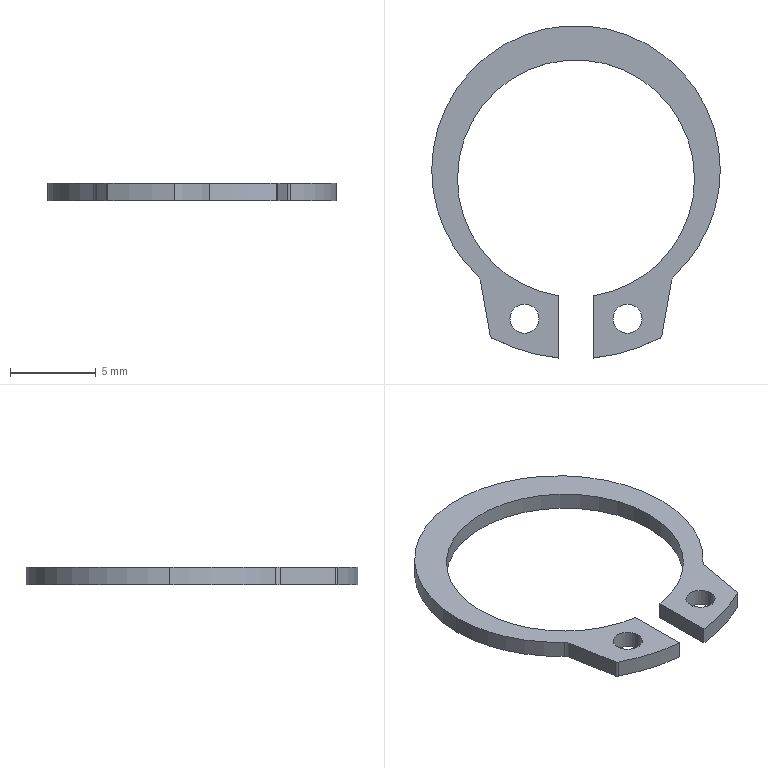Part | SolidWorks | features Extrusion 1 | 1 solid | 22 faces | box 16.8 x 19.352 x 1 mm | volume 89.212 mm3 | cylinder 16 | plane 6 | commonest cylinder face diameters 1.7 x4 13.8 x3 16.8 x3 0.4 x2 1 x2 21 x2
STEP:
#1=CARTESIAN_POINT('',(2.15,-8.666,0.5));
#2=VERTEX_POINT('',#1);
#3=CARTESIAN_POINT('',(3.85,-8.666,0.5));
#4=VERTEX_POINT('',#3);
#5=CARTESIAN_POINT('',(3.,-8.666,0.5));
#6=DIRECTION('',(0.,0.,1.));
#7=DIRECTION('',(-1.,0.,0.));
#8=AXIS2_PLACEMENT_3D('',#5,#6,#7);
#9=CIRCLE('',#8,0.85);
#10=EDGE_CURVE('',#2,#4,#9,.T.);
#11=ORIENTED_EDGE('',*,*,#10,.T.);
#12=CARTESIAN_POINT('',(3.85,-8.666,-0.5));
#13=VERTEX_POINT('',#12);
#14=CARTESIAN_POINT('',(3.85,-8.666,0.5));
#15=DIRECTION('',(0.,0.,-1.));
#16=VECTOR('',#15,1000.);
#17=LINE('',#14,#16);
#18=EDGE_CURVE('',#4,#13,#17,.T.);
#19=ORIENTED_EDGE('',*,*,#18,.T.);
#20=CARTESIAN_POINT('',(2.15,-8.666,-0.5));
#21=VERTEX_POINT('',#20);
#22=CARTESIAN_POINT('',(3.,-8.666,-0.5));
#23=DIRECTION('',(0.,0.,1.));
#24=DIRECTION('',(-1.,0.,0.));
#25=AXIS2_PLACEMENT_3D('',#22,#23,#24);
#26=CIRCLE('',#25,0.85);
#27=EDGE_CURVE('',#21,#13,#26,.T.);
#28=ORIENTED_EDGE('',*,*,#27,.F.);
#29=CARTESIAN_POINT('',(2.15,-8.666,0.5));
#30=DIRECTION('',(0.,0.,-1.));
#31=VECTOR('',#30,1000.);
#32=LINE('',#29,#31);
#33=EDGE_CURVE('',#2,#21,#32,.T.);
#34=ORIENTED_EDGE('',*,*,#33,.F.);
#35=EDGE_LOOP('',(#11,#19,#28,#34));
#36=FACE_OUTER_BOUND('',#35,.T.);
#37=CARTESIAN_POINT('',(3.,-8.666,0.5));
#38=DIRECTION('',(0.,0.,-1.));
#39=DIRECTION('',(-1.,0.,0.));
#40=AXIS2_PLACEMENT_3D('',#37,#38,#39);
#41=CYLINDRICAL_SURFACE('',#40,0.85);
#42=ADVANCED_FACE('',(#36),#41,.F.);
#43=CARTESIAN_POINT('',(-3.85,-8.666,0.5));
#44=VERTEX_POINT('',#43);
#45=CARTESIAN_POINT('',(-2.15,-8.666,0.5));
#46=VERTEX_POINT('',#45);
#47=CARTESIAN_POINT('',(-3.,-8.666,0.5));
#48=DIRECTION('',(0.,0.,1.));
#49=DIRECTION('',(1.,0.,0.));
#50=AXIS2_PLACEMENT_3D('',#47,#48,#49);
#51=CIRCLE('',#50,0.85);
#52=EDGE_CURVE('',#44,#46,#51,.T.);
#53=ORIENTED_EDGE('',*,*,#52,.T.);
#54=CARTESIAN_POINT('',(-2.15,-8.666,-0.5));
#55=VERTEX_POINT('',#54);
#56=CARTESIAN_POINT('',(-2.15,-8.666,0.5));
#57=DIRECTION('',(0.,0.,-1.));
#58=VECTOR('',#57,1000.);
#59=LINE('',#56,#58);
#60=EDGE_CURVE('',#46,#55,#59,.T.);
#61=ORIENTED_EDGE('',*,*,#60,.T.);
#62=CARTESIAN_POINT('',(-3.85,-8.666,-0.5));
#63=VERTEX_POINT('',#62);
#64=CARTESIAN_POINT('',(-3.,-8.666,-0.5));
#65=DIRECTION('',(0.,0.,1.));
#66=DIRECTION('',(1.,0.,0.));
#67=AXIS2_PLACEMENT_3D('',#64,#65,#66);
#68=CIRCLE('',#67,0.85);
#69=EDGE_CURVE('',#63,#55,#68,.T.);
#70=ORIENTED_EDGE('',*,*,#69,.F.);
#71=CARTESIAN_POINT('',(-3.85,-8.666,0.5));
#72=DIRECTION('',(0.,0.,-1.));
#73=VECTOR('',#72,1000.);
#74=LINE('',#71,#73);
#75=EDGE_CURVE('',#44,#63,#74,.T.);
#76=ORIENTED_EDGE('',*,*,#75,.F.);
#77=EDGE_LOOP('',(#53,#61,#70,#76));
#78=FACE_OUTER_BOUND('',#77,.T.);
#79=CARTESIAN_POINT('',(-3.,-8.666,0.5));
#80=DIRECTION('',(0.,0.,-1.));
#81=DIRECTION('',(-1.,0.,0.));
#82=AXIS2_PLACEMENT_3D('',#79,#80,#81);
#83=CYLINDRICAL_SURFACE('',#82,0.85);
#84=ADVANCED_FACE('',(#78),#83,.F.);
#85=CARTESIAN_POINT('',(8.4,0.,0.5));
#86=VERTEX_POINT('',#85);
#87=CARTESIAN_POINT('',(-8.4,0.,0.5));
#88=VERTEX_POINT('',#87);
#89=CARTESIAN_POINT('',(0.,0.,0.5));
#90=DIRECTION('',(0.,0.,1.));
#91=DIRECTION('',(1.,0.,0.));
#92=AXIS2_PLACEMENT_3D('',#89,#90,#91);
#93=CIRCLE('',#92,8.4);
#94=EDGE_CURVE('',#86,#88,#93,.T.);
#95=ORIENTED_EDGE('',*,*,#94,.F.);
#96=CARTESIAN_POINT('',(8.4,0.,-0.5));
#97=VERTEX_POINT('',#96);
#98=CARTESIAN_POINT('',(8.4,0.,0.5));
#99=DIRECTION('',(0.,0.,-1.));
#100=VECTOR('',#99,1000.);
#101=LINE('',#98,#100);
#102=EDGE_CURVE('',#86,#97,#101,.T.);
#103=ORIENTED_EDGE('',*,*,#102,.T.);
#104=CARTESIAN_POINT('',(-8.4,0.,-0.5));
#105=VERTEX_POINT('',#104);
#106=CARTESIAN_POINT('',(0.,0.,-0.5));
#107=DIRECTION('',(0.,0.,1.));
#108=DIRECTION('',(1.,0.,0.));
#109=AXIS2_PLACEMENT_3D('',#106,#107,#108);
#110=CIRCLE('',#109,8.4);
#111=EDGE_CURVE('',#97,#105,#110,.T.);
#112=ORIENTED_EDGE('',*,*,#111,.T.);
#113=CARTESIAN_POINT('',(-8.4,0.,0.5));
#114=DIRECTION('',(0.,0.,-1.));
#115=VECTOR('',#114,1000.);
#116=LINE('',#113,#115);
#117=EDGE_CURVE('',#88,#105,#116,.T.);
#118=ORIENTED_EDGE('',*,*,#117,.F.);
#119=EDGE_LOOP('',(#95,#103,#112,#118));
#120=FACE_OUTER_BOUND('',#119,.T.);
#121=CARTESIAN_POINT('',(0.,0.,0.5));
#122=DIRECTION('',(0.,0.,-1.));
#123=DIRECTION('',(-1.,0.,0.));
#124=AXIS2_PLACEMENT_3D('',#121,#122,#123);
#125=CYLINDRICAL_SURFACE('',#124,8.4);
#126=ADVANCED_FACE('',(#120),#125,.T.);
#127=CARTESIAN_POINT('',(-5.719,-6.153,0.5));
#128=VERTEX_POINT('',#127);
#129=CARTESIAN_POINT('',(0.,0.,0.5));
#130=DIRECTION('',(0.,0.,1.));
#131=DIRECTION('',(1.,0.,0.));
#132=AXIS2_PLACEMENT_3D('',#129,#130,#131);
#133=CIRCLE('',#132,8.4);
#134=EDGE_CURVE('',#88,#128,#133,.T.);
#135=ORIENTED_EDGE('',*,*,#134,.F.);
#136=ORIENTED_EDGE('',*,*,#117,.T.);
#137=CARTESIAN_POINT('',(-5.719,-6.153,-0.5));
#138=VERTEX_POINT('',#137);
#139=CARTESIAN_POINT('',(0.,0.,-0.5));
#140=DIRECTION('',(0.,0.,1.));
#141=DIRECTION('',(1.,0.,0.));
#142=AXIS2_PLACEMENT_3D('',#139,#140,#141);
#143=CIRCLE('',#142,8.4);
#144=EDGE_CURVE('',#105,#138,#143,.T.);
#145=ORIENTED_EDGE('',*,*,#144,.T.);
#146=CARTESIAN_POINT('',(-5.719,-6.153,0.5));
#147=DIRECTION('',(0.,0.,-1.));
#148=VECTOR('',#147,1000.);
#149=LINE('',#146,#148);
#150=EDGE_CURVE('',#128,#138,#149,.T.);
#151=ORIENTED_EDGE('',*,*,#150,.F.);
#152=EDGE_LOOP('',(#135,#136,#145,#151));
#153=FACE_OUTER_BOUND('',#152,.T.);
#154=CARTESIAN_POINT('',(0.,0.,0.5));
#155=DIRECTION('',(0.,0.,-1.));
#156=DIRECTION('',(-1.,0.,0.));
#157=AXIS2_PLACEMENT_3D('',#154,#155,#156);
#158=CYLINDRICAL_SURFACE('',#157,8.4);
#159=ADVANCED_FACE('',(#153),#158,.T.);
#160=CARTESIAN_POINT('',(6.9,-0.5,0.5));
#161=VERTEX_POINT('',#160);
#162=CARTESIAN_POINT('',(1.,-7.327,0.5));
#163=VERTEX_POINT('',#162);
#164=CARTESIAN_POINT('',(0.,-0.5,0.5));
#165=DIRECTION('',(0.,0.,-1.));
#166=DIRECTION('',(1.,0.,0.));
#167=AXIS2_PLACEMENT_3D('',#164,#165,#166);
#168=CIRCLE('',#167,6.9);
#169=EDGE_CURVE('',#161,#163,#168,.T.);
#170=ORIENTED_EDGE('',*,*,#169,.F.);
#171=CARTESIAN_POINT('',(6.9,-0.5,-0.5));
#172=VERTEX_POINT('',#171);
#173=CARTESIAN_POINT('',(6.9,-0.5,0.5));
#174=DIRECTION('',(0.,0.,-1.));
#175=VECTOR('',#174,1000.);
#176=LINE('',#173,#175);
#177=EDGE_CURVE('',#161,#172,#176,.T.);
#178=ORIENTED_EDGE('',*,*,#177,.T.);
#179=CARTESIAN_POINT('',(1.,-7.327,-0.5));
#180=VERTEX_POINT('',#179);
#181=CARTESIAN_POINT('',(0.,-0.5,-0.5));
#182=DIRECTION('',(0.,0.,-1.));
#183=DIRECTION('',(1.,0.,0.));
#184=AXIS2_PLACEMENT_3D('',#181,#182,#183);
#185=CIRCLE('',#184,6.9);
#186=EDGE_CURVE('',#172,#180,#185,.T.);
#187=ORIENTED_EDGE('',*,*,#186,.T.);
#188=CARTESIAN_POINT('',(1.,-7.327,0.5));
#189=DIRECTION('',(0.,0.,-1.));
#190=VECTOR('',#189,1000.);
#191=LINE('',#188,#190);
#192=EDGE_CURVE('',#163,#180,#191,.T.);
#193=ORIENTED_EDGE('',*,*,#192,.F.);
#194=EDGE_LOOP('',(#170,#178,#187,#193));
#195=FACE_OUTER_BOUND('',#194,.T.);
#196=CARTESIAN_POINT('',(0.,-0.5,0.5));
#197=DIRECTION('',(0.,0.,-1.));
#198=DIRECTION('',(-1.,0.,0.));
#199=AXIS2_PLACEMENT_3D('',#196,#197,#198);
#200=CYLINDRICAL_SURFACE('',#199,6.9);
#201=ADVANCED_FACE('',(#195),#200,.F.);
#202=ORIENTED_EDGE('',*,*,#177,.F.);
#203=CARTESIAN_POINT('',(-6.9,-0.5,0.5));
#204=VERTEX_POINT('',#203);
#205=CARTESIAN_POINT('',(0.,-0.5,0.5));
#206=DIRECTION('',(0.,0.,-1.));
#207=DIRECTION('',(1.,0.,0.));
#208=AXIS2_PLACEMENT_3D('',#205,#206,#207);
#209=CIRCLE('',#208,6.9);
#210=EDGE_CURVE('',#204,#161,#209,.T.);
#211=ORIENTED_EDGE('',*,*,#210,.F.);
#212=CARTESIAN_POINT('',(-6.9,-0.5,-0.5));
#213=VERTEX_POINT('',#212);
#214=CARTESIAN_POINT('',(-6.9,-0.5,0.5));
#215=DIRECTION('',(0.,0.,-1.));
#216=VECTOR('',#215,1000.);
#217=LINE('',#214,#216);
#218=EDGE_CURVE('',#204,#213,#217,.T.);
#219=ORIENTED_EDGE('',*,*,#218,.T.);
#220=CARTESIAN_POINT('',(0.,-0.5,-0.5));
#221=DIRECTION('',(0.,0.,-1.));
#222=DIRECTION('',(1.,0.,0.));
#223=AXIS2_PLACEMENT_3D('',#220,#221,#222);
#224=CIRCLE('',#223,6.9);
#225=EDGE_CURVE('',#213,#172,#224,.T.);
#226=ORIENTED_EDGE('',*,*,#225,.T.);
#227=EDGE_LOOP('',(#202,#211,#219,#226));
#228=FACE_OUTER_BOUND('',#227,.T.);
#229=CARTESIAN_POINT('',(0.,-0.5,0.5));
#230=DIRECTION('',(0.,0.,-1.));
#231=DIRECTION('',(-1.,0.,0.));
#232=AXIS2_PLACEMENT_3D('',#229,#230,#231);
#233=CYLINDRICAL_SURFACE('',#232,6.9);
#234=ADVANCED_FACE('',(#228),#233,.F.);
#235=ORIENTED_EDGE('',*,*,#52,.F.);
#236=CARTESIAN_POINT('',(-3.,-8.666,0.5));
#237=DIRECTION('',(0.,0.,1.));
#238=DIRECTION('',(1.,0.,0.));
#239=AXIS2_PLACEMENT_3D('',#236,#237,#238);
#240=CIRCLE('',#239,0.85);
#241=EDGE_CURVE('',#46,#44,#240,.T.);
#242=ORIENTED_EDGE('',*,*,#241,.F.);
#243=EDGE_LOOP('',(#235,#242));
#244=FACE_BOUND('',#243,.T.);
#245=CARTESIAN_POINT('',(-5.567,-6.432,0.5));
#246=VERTEX_POINT('',#245);
#247=CARTESIAN_POINT('',(-6.059,-6.519,0.5));
#248=DIRECTION('',(0.,0.,-1.));
#249=DIRECTION('',(1.,0.,0.));
#250=AXIS2_PLACEMENT_3D('',#247,#248,#249);
#251=CIRCLE('',#250,0.5);
#252=EDGE_CURVE('',#128,#246,#251,.T.);
#253=ORIENTED_EDGE('',*,*,#252,.T.);
#254=CARTESIAN_POINT('',(-5.,-9.646,0.5));
#255=VERTEX_POINT('',#254);
#256=CARTESIAN_POINT('',(-5.567,-6.432,0.5));
#257=DIRECTION('',(0.1736,-0.9848,0.));
#258=VECTOR('',#257,1000.);
#259=LINE('',#256,#258);
#260=EDGE_CURVE('',#246,#255,#259,.T.);
#261=ORIENTED_EDGE('',*,*,#260,.T.);
#262=CARTESIAN_POINT('',(-4.896,-9.789,0.5));
#263=VERTEX_POINT('',#262);
#264=CARTESIAN_POINT('',(-4.803,-9.612,0.5));
#265=DIRECTION('',(0.,0.,1.));
#266=DIRECTION('',(-1.,0.,0.));
#267=AXIS2_PLACEMENT_3D('',#264,#265,#266);
#268=CIRCLE('',#267,0.2);
#269=EDGE_CURVE('',#255,#263,#268,.T.);
#270=ORIENTED_EDGE('',*,*,#269,.T.);
#271=CARTESIAN_POINT('',(-1.,-10.952,0.5));
#272=VERTEX_POINT('',#271);
#273=CARTESIAN_POINT('',(0.,-0.5,0.5));
#274=DIRECTION('',(0.,0.,1.));
#275=DIRECTION('',(-1.,0.,0.));
#276=AXIS2_PLACEMENT_3D('',#273,#274,#275);
#277=CIRCLE('',#276,10.5);
#278=EDGE_CURVE('',#263,#272,#277,.T.);
#279=ORIENTED_EDGE('',*,*,#278,.T.);
#280=CARTESIAN_POINT('',(-1.,-7.327,0.5));
#281=VERTEX_POINT('',#280);
#282=CARTESIAN_POINT('',(-1.,-7.327,0.5));
#283=DIRECTION('',(0.,1.,0.));
#284=VECTOR('',#283,1000.);
#285=LINE('',#282,#284);
#286=EDGE_CURVE('',#272,#281,#285,.T.);
#287=ORIENTED_EDGE('',*,*,#286,.T.);
#288=CARTESIAN_POINT('',(0.,-0.5,0.5));
#289=DIRECTION('',(0.,0.,-1.));
#290=DIRECTION('',(1.,0.,0.));
#291=AXIS2_PLACEMENT_3D('',#288,#289,#290);
#292=CIRCLE('',#291,6.9);
#293=EDGE_CURVE('',#281,#204,#292,.T.);
#294=ORIENTED_EDGE('',*,*,#293,.T.);
#295=ORIENTED_EDGE('',*,*,#210,.T.);
#296=ORIENTED_EDGE('',*,*,#169,.T.);
#297=CARTESIAN_POINT('',(1.,-10.952,0.5));
#298=VERTEX_POINT('',#297);
#299=CARTESIAN_POINT('',(1.,-7.327,0.5));
#300=DIRECTION('',(0.,-1.,0.));
#301=VECTOR('',#300,1000.);
#302=LINE('',#299,#301);
#303=EDGE_CURVE('',#163,#298,#302,.T.);
#304=ORIENTED_EDGE('',*,*,#303,.T.);
#305=CARTESIAN_POINT('',(4.896,-9.789,0.5));
#306=VERTEX_POINT('',#305);
#307=CARTESIAN_POINT('',(0.,-0.5,0.5));
#308=DIRECTION('',(0.,0.,1.));
#309=DIRECTION('',(1.,0.,0.));
#310=AXIS2_PLACEMENT_3D('',#307,#308,#309);
#311=CIRCLE('',#310,10.5);
#312=EDGE_CURVE('',#298,#306,#311,.T.);
#313=ORIENTED_EDGE('',*,*,#312,.T.);
#314=CARTESIAN_POINT('',(5.,-9.646,0.5));
#315=VERTEX_POINT('',#314);
#316=CARTESIAN_POINT('',(4.803,-9.612,0.5));
#317=DIRECTION('',(0.,0.,1.));
#318=DIRECTION('',(1.,0.,0.));
#319=AXIS2_PLACEMENT_3D('',#316,#317,#318);
#320=CIRCLE('',#319,0.2);
#321=EDGE_CURVE('',#306,#315,#320,.T.);
#322=ORIENTED_EDGE('',*,*,#321,.T.);
#323=CARTESIAN_POINT('',(5.567,-6.432,0.5));
#324=VERTEX_POINT('',#323);
#325=CARTESIAN_POINT('',(5.567,-6.432,0.5));
#326=DIRECTION('',(0.1736,0.9848,0.));
#327=VECTOR('',#326,1000.);
#328=LINE('',#325,#327);
#329=EDGE_CURVE('',#315,#324,#328,.T.);
#330=ORIENTED_EDGE('',*,*,#329,.T.);
#331=CARTESIAN_POINT('',(5.719,-6.153,0.5));
#332=VERTEX_POINT('',#331);
#333=CARTESIAN_POINT('',(6.059,-6.519,0.5));
#334=DIRECTION('',(0.,0.,-1.));
#335=DIRECTION('',(-1.,0.,0.));
#336=AXIS2_PLACEMENT_3D('',#333,#334,#335);
#337=CIRCLE('',#336,0.5);
#338=EDGE_CURVE('',#324,#332,#337,.T.);
#339=ORIENTED_EDGE('',*,*,#338,.T.);
#340=CARTESIAN_POINT('',(0.,0.,0.5));
#341=DIRECTION('',(0.,0.,1.));
#342=DIRECTION('',(1.,0.,0.));
#343=AXIS2_PLACEMENT_3D('',#340,#341,#342);
#344=CIRCLE('',#343,8.4);
#345=EDGE_CURVE('',#332,#86,#344,.T.);
#346=ORIENTED_EDGE('',*,*,#345,.T.);
#347=ORIENTED_EDGE('',*,*,#94,.T.);
#348=ORIENTED_EDGE('',*,*,#134,.T.);
#349=EDGE_LOOP('',(#253,#261,#270,#279,#287,#294,#295,#296,#304,#313,#322,#330,#339,#346,#347,#348));
#350=FACE_OUTER_BOUND('',#349,.T.);
#351=ORIENTED_EDGE('',*,*,#10,.F.);
#352=CARTESIAN_POINT('',(3.,-8.666,0.5));
#353=DIRECTION('',(0.,0.,1.));
#354=DIRECTION('',(-1.,0.,0.));
#355=AXIS2_PLACEMENT_3D('',#352,#353,#354);
#356=CIRCLE('',#355,0.85);
#357=EDGE_CURVE('',#4,#2,#356,.T.);
#358=ORIENTED_EDGE('',*,*,#357,.F.);
#359=EDGE_LOOP('',(#351,#358));
#360=FACE_BOUND('',#359,.T.);
#361=CARTESIAN_POINT('',(-6.059,-6.519,0.5));
#362=DIRECTION('',(0.,0.,1.));
#363=DIRECTION('',(1.,0.,0.));
#364=AXIS2_PLACEMENT_3D('',#361,#362,#363);
#365=PLANE('',#364);
#366=ADVANCED_FACE('',(#244,#350,#360),#365,.T.);
#367=ORIENTED_EDGE('',*,*,#150,.T.);
#368=CARTESIAN_POINT('',(-5.567,-6.432,-0.5));
#369=VERTEX_POINT('',#368);
#370=CARTESIAN_POINT('',(-6.059,-6.519,-0.5));
#371=DIRECTION('',(0.,0.,-1.));
#372=DIRECTION('',(1.,0.,0.));
#373=AXIS2_PLACEMENT_3D('',#370,#371,#372);
#374=CIRCLE('',#373,0.5);
#375=EDGE_CURVE('',#138,#369,#374,.T.);
#376=ORIENTED_EDGE('',*,*,#375,.T.);
#377=CARTESIAN_POINT('',(-5.567,-6.432,0.5));
#378=DIRECTION('',(0.,0.,-1.));
#379=VECTOR('',#378,1000.);
#380=LINE('',#377,#379);
#381=EDGE_CURVE('',#246,#369,#380,.T.);
#382=ORIENTED_EDGE('',*,*,#381,.F.);
#383=ORIENTED_EDGE('',*,*,#252,.F.);
#384=EDGE_LOOP('',(#367,#376,#382,#383));
#385=FACE_OUTER_BOUND('',#384,.T.);
#386=CARTESIAN_POINT('',(-6.059,-6.519,0.5));
#387=DIRECTION('',(0.,0.,-1.));
#388=DIRECTION('',(-1.,0.,0.));
#389=AXIS2_PLACEMENT_3D('',#386,#387,#388);
#390=CYLINDRICAL_SURFACE('',#389,0.5);
#391=ADVANCED_FACE('',(#385),#390,.F.);
#392=ORIENTED_EDGE('',*,*,#381,.T.);
#393=CARTESIAN_POINT('',(-5.,-9.646,-0.5));
#394=VERTEX_POINT('',#393);
#395=CARTESIAN_POINT('',(-5.567,-6.432,-0.5));
#396=DIRECTION('',(0.1736,-0.9848,0.));
#397=VECTOR('',#396,1000.);
#398=LINE('',#395,#397);
#399=EDGE_CURVE('',#369,#394,#398,.T.);
#400=ORIENTED_EDGE('',*,*,#399,.T.);
#401=CARTESIAN_POINT('',(-5.,-9.646,0.5));
#402=DIRECTION('',(0.,0.,-1.));
#403=VECTOR('',#402,1000.);
#404=LINE('',#401,#403);
#405=EDGE_CURVE('',#255,#394,#404,.T.);
#406=ORIENTED_EDGE('',*,*,#405,.F.);
#407=ORIENTED_EDGE('',*,*,#260,.F.);
#408=EDGE_LOOP('',(#392,#400,#406,#407));
#409=FACE_OUTER_BOUND('',#408,.T.);
#410=CARTESIAN_POINT('',(-5.567,-6.432,0.5));
#411=DIRECTION('',(0.9848,0.1736,0.));
#412=DIRECTION('',(-0.1736,0.9848,0.));
#413=AXIS2_PLACEMENT_3D('',#410,#411,#412);
#414=PLANE('',#413);
#415=ADVANCED_FACE('',(#409),#414,.F.);
#416=ORIENTED_EDGE('',*,*,#405,.T.);
#417=CARTESIAN_POINT('',(-4.896,-9.789,-0.5));
#418=VERTEX_POINT('',#417);
#419=CARTESIAN_POINT('',(-4.803,-9.612,-0.5));
#420=DIRECTION('',(0.,0.,1.));
#421=DIRECTION('',(-1.,0.,0.));
#422=AXIS2_PLACEMENT_3D('',#419,#420,#421);
#423=CIRCLE('',#422,0.2);
#424=EDGE_CURVE('',#394,#418,#423,.T.);
#425=ORIENTED_EDGE('',*,*,#424,.T.);
#426=CARTESIAN_POINT('',(-4.896,-9.789,0.5));
#427=DIRECTION('',(0.,0.,-1.));
#428=VECTOR('',#427,1000.);
#429=LINE('',#426,#428);
#430=EDGE_CURVE('',#263,#418,#429,.T.);
#431=ORIENTED_EDGE('',*,*,#430,.F.);
#432=ORIENTED_EDGE('',*,*,#269,.F.);
#433=EDGE_LOOP('',(#416,#425,#431,#432));
#434=FACE_OUTER_BOUND('',#433,.T.);
#435=CARTESIAN_POINT('',(-4.803,-9.612,0.5));
#436=DIRECTION('',(0.,0.,-1.));
#437=DIRECTION('',(-1.,0.,0.));
#438=AXIS2_PLACEMENT_3D('',#435,#436,#437);
#439=CYLINDRICAL_SURFACE('',#438,0.2);
#440=ADVANCED_FACE('',(#434),#439,.T.);
#441=ORIENTED_EDGE('',*,*,#430,.T.);
#442=CARTESIAN_POINT('',(-1.,-10.952,-0.5));
#443=VERTEX_POINT('',#442);
#444=CARTESIAN_POINT('',(0.,-0.5,-0.5));
#445=DIRECTION('',(0.,0.,1.));
#446=DIRECTION('',(-1.,0.,0.));
#447=AXIS2_PLACEMENT_3D('',#444,#445,#446);
#448=CIRCLE('',#447,10.5);
#449=EDGE_CURVE('',#418,#443,#448,.T.);
#450=ORIENTED_EDGE('',*,*,#449,.T.);
#451=CARTESIAN_POINT('',(-1.,-10.952,0.5));
#452=DIRECTION('',(0.,0.,-1.));
#453=VECTOR('',#452,1000.);
#454=LINE('',#451,#453);
#455=EDGE_CURVE('',#272,#443,#454,.T.);
#456=ORIENTED_EDGE('',*,*,#455,.F.);
#457=ORIENTED_EDGE('',*,*,#278,.F.);
#458=EDGE_LOOP('',(#441,#450,#456,#457));
#459=FACE_OUTER_BOUND('',#458,.T.);
#460=CARTESIAN_POINT('',(0.,-0.5,0.5));
#461=DIRECTION('',(0.,0.,-1.));
#462=DIRECTION('',(-1.,0.,0.));
#463=AXIS2_PLACEMENT_3D('',#460,#461,#462);
#464=CYLINDRICAL_SURFACE('',#463,10.5);
#465=ADVANCED_FACE('',(#459),#464,.T.);
#466=ORIENTED_EDGE('',*,*,#455,.T.);
#467=CARTESIAN_POINT('',(-1.,-7.327,-0.5));
#468=VERTEX_POINT('',#467);
#469=CARTESIAN_POINT('',(-1.,-7.327,-0.5));
#470=DIRECTION('',(0.,1.,0.));
#471=VECTOR('',#470,1000.);
#472=LINE('',#469,#471);
#473=EDGE_CURVE('',#443,#468,#472,.T.);
#474=ORIENTED_EDGE('',*,*,#473,.T.);
#475=CARTESIAN_POINT('',(-1.,-7.327,0.5));
#476=DIRECTION('',(0.,0.,-1.));
#477=VECTOR('',#476,1000.);
#478=LINE('',#475,#477);
#479=EDGE_CURVE('',#281,#468,#478,.T.);
#480=ORIENTED_EDGE('',*,*,#479,.F.);
#481=ORIENTED_EDGE('',*,*,#286,.F.);
#482=EDGE_LOOP('',(#466,#474,#480,#481));
#483=FACE_OUTER_BOUND('',#482,.T.);
#484=CARTESIAN_POINT('',(-1.,-7.327,0.5));
#485=DIRECTION('',(-1.,0.,0.));
#486=DIRECTION('',(0.,-1.,0.));
#487=AXIS2_PLACEMENT_3D('',#484,#485,#486);
#488=PLANE('',#487);
#489=ADVANCED_FACE('',(#483),#488,.F.);
#490=ORIENTED_EDGE('',*,*,#218,.F.);
#491=ORIENTED_EDGE('',*,*,#293,.F.);
#492=ORIENTED_EDGE('',*,*,#479,.T.);
#493=CARTESIAN_POINT('',(0.,-0.5,-0.5));
#494=DIRECTION('',(0.,0.,-1.));
#495=DIRECTION('',(1.,0.,0.));
#496=AXIS2_PLACEMENT_3D('',#493,#494,#495);
#497=CIRCLE('',#496,6.9);
#498=EDGE_CURVE('',#468,#213,#497,.T.);
#499=ORIENTED_EDGE('',*,*,#498,.T.);
#500=EDGE_LOOP('',(#490,#491,#492,#499));
#501=FACE_OUTER_BOUND('',#500,.T.);
#502=CARTESIAN_POINT('',(0.,-0.5,0.5));
#503=DIRECTION('',(0.,0.,-1.));
#504=DIRECTION('',(-1.,0.,0.));
#505=AXIS2_PLACEMENT_3D('',#502,#503,#504);
#506=CYLINDRICAL_SURFACE('',#505,6.9);
#507=ADVANCED_FACE('',(#501),#506,.F.);
#508=ORIENTED_EDGE('',*,*,#192,.T.);
#509=CARTESIAN_POINT('',(1.,-10.952,-0.5));
#510=VERTEX_POINT('',#509);
#511=CARTESIAN_POINT('',(1.,-7.327,-0.5));
#512=DIRECTION('',(0.,-1.,0.));
#513=VECTOR('',#512,1000.);
#514=LINE('',#511,#513);
#515=EDGE_CURVE('',#180,#510,#514,.T.);
#516=ORIENTED_EDGE('',*,*,#515,.T.);
#517=CARTESIAN_POINT('',(1.,-10.952,0.5));
#518=DIRECTION('',(0.,0.,-1.));
#519=VECTOR('',#518,1000.);
#520=LINE('',#517,#519);
#521=EDGE_CURVE('',#298,#510,#520,.T.);
#522=ORIENTED_EDGE('',*,*,#521,.F.);
#523=ORIENTED_EDGE('',*,*,#303,.F.);
#524=EDGE_LOOP('',(#508,#516,#522,#523));
#525=FACE_OUTER_BOUND('',#524,.T.);
#526=CARTESIAN_POINT('',(1.,-7.327,0.5));
#527=DIRECTION('',(1.,0.,0.));
#528=DIRECTION('',(0.,1.,0.));
#529=AXIS2_PLACEMENT_3D('',#526,#527,#528);
#530=PLANE('',#529);
#531=ADVANCED_FACE('',(#525),#530,.F.);
#532=ORIENTED_EDGE('',*,*,#521,.T.);
#533=CARTESIAN_POINT('',(4.896,-9.789,-0.5));
#534=VERTEX_POINT('',#533);
#535=CARTESIAN_POINT('',(0.,-0.5,-0.5));
#536=DIRECTION('',(0.,0.,1.));
#537=DIRECTION('',(1.,0.,0.));
#538=AXIS2_PLACEMENT_3D('',#535,#536,#537);
#539=CIRCLE('',#538,10.5);
#540=EDGE_CURVE('',#510,#534,#539,.T.);
#541=ORIENTED_EDGE('',*,*,#540,.T.);
#542=CARTESIAN_POINT('',(4.896,-9.789,0.5));
#543=DIRECTION('',(0.,0.,-1.));
#544=VECTOR('',#543,1000.);
#545=LINE('',#542,#544);
#546=EDGE_CURVE('',#306,#534,#545,.T.);
#547=ORIENTED_EDGE('',*,*,#546,.F.);
#548=ORIENTED_EDGE('',*,*,#312,.F.);
#549=EDGE_LOOP('',(#532,#541,#547,#548));
#550=FACE_OUTER_BOUND('',#549,.T.);
#551=CARTESIAN_POINT('',(0.,-0.5,0.5));
#552=DIRECTION('',(0.,0.,-1.));
#553=DIRECTION('',(-1.,0.,0.));
#554=AXIS2_PLACEMENT_3D('',#551,#552,#553);
#555=CYLINDRICAL_SURFACE('',#554,10.5);
#556=ADVANCED_FACE('',(#550),#555,.T.);
#557=ORIENTED_EDGE('',*,*,#546,.T.);
#558=CARTESIAN_POINT('',(5.,-9.646,-0.5));
#559=VERTEX_POINT('',#558);
#560=CARTESIAN_POINT('',(4.803,-9.612,-0.5));
#561=DIRECTION('',(0.,0.,1.));
#562=DIRECTION('',(1.,0.,0.));
#563=AXIS2_PLACEMENT_3D('',#560,#561,#562);
#564=CIRCLE('',#563,0.2);
#565=EDGE_CURVE('',#534,#559,#564,.T.);
#566=ORIENTED_EDGE('',*,*,#565,.T.);
#567=CARTESIAN_POINT('',(5.,-9.646,0.5));
#568=DIRECTION('',(0.,0.,-1.));
#569=VECTOR('',#568,1000.);
#570=LINE('',#567,#569);
#571=EDGE_CURVE('',#315,#559,#570,.T.);
#572=ORIENTED_EDGE('',*,*,#571,.F.);
#573=ORIENTED_EDGE('',*,*,#321,.F.);
#574=EDGE_LOOP('',(#557,#566,#572,#573));
#575=FACE_OUTER_BOUND('',#574,.T.);
#576=CARTESIAN_POINT('',(4.803,-9.612,0.5));
#577=DIRECTION('',(0.,0.,-1.));
#578=DIRECTION('',(-1.,0.,0.));
#579=AXIS2_PLACEMENT_3D('',#576,#577,#578);
#580=CYLINDRICAL_SURFACE('',#579,0.2);
#581=ADVANCED_FACE('',(#575),#580,.T.);
#582=ORIENTED_EDGE('',*,*,#571,.T.);
#583=CARTESIAN_POINT('',(5.567,-6.432,-0.5));
#584=VERTEX_POINT('',#583);
#585=CARTESIAN_POINT('',(5.567,-6.432,-0.5));
#586=DIRECTION('',(0.1736,0.9848,0.));
#587=VECTOR('',#586,1000.);
#588=LINE('',#585,#587);
#589=EDGE_CURVE('',#559,#584,#588,.T.);
#590=ORIENTED_EDGE('',*,*,#589,.T.);
#591=CARTESIAN_POINT('',(5.567,-6.432,0.5));
#592=DIRECTION('',(0.,0.,-1.));
#593=VECTOR('',#592,1000.);
#594=LINE('',#591,#593);
#595=EDGE_CURVE('',#324,#584,#594,.T.);
#596=ORIENTED_EDGE('',*,*,#595,.F.);
#597=ORIENTED_EDGE('',*,*,#329,.F.);
#598=EDGE_LOOP('',(#582,#590,#596,#597));
#599=FACE_OUTER_BOUND('',#598,.T.);
#600=CARTESIAN_POINT('',(5.567,-6.432,0.5));
#601=DIRECTION('',(-0.9848,0.1736,0.));
#602=DIRECTION('',(-0.1736,-0.9848,0.));
#603=AXIS2_PLACEMENT_3D('',#600,#601,#602);
#604=PLANE('',#603);
#605=ADVANCED_FACE('',(#599),#604,.F.);
#606=ORIENTED_EDGE('',*,*,#595,.T.);
#607=CARTESIAN_POINT('',(5.719,-6.153,-0.5));
#608=VERTEX_POINT('',#607);
#609=CARTESIAN_POINT('',(6.059,-6.519,-0.5));
#610=DIRECTION('',(0.,0.,-1.));
#611=DIRECTION('',(-1.,0.,0.));
#612=AXIS2_PLACEMENT_3D('',#609,#610,#611);
#613=CIRCLE('',#612,0.5);
#614=EDGE_CURVE('',#584,#608,#613,.T.);
#615=ORIENTED_EDGE('',*,*,#614,.T.);
#616=CARTESIAN_POINT('',(5.719,-6.153,0.5));
#617=DIRECTION('',(0.,0.,-1.));
#618=VECTOR('',#617,1000.);
#619=LINE('',#616,#618);
#620=EDGE_CURVE('',#332,#608,#619,.T.);
#621=ORIENTED_EDGE('',*,*,#620,.F.);
#622=ORIENTED_EDGE('',*,*,#338,.F.);
#623=EDGE_LOOP('',(#606,#615,#621,#622));
#624=FACE_OUTER_BOUND('',#623,.T.);
#625=CARTESIAN_POINT('',(6.059,-6.519,0.5));
#626=DIRECTION('',(0.,0.,-1.));
#627=DIRECTION('',(-1.,0.,0.));
#628=AXIS2_PLACEMENT_3D('',#625,#626,#627);
#629=CYLINDRICAL_SURFACE('',#628,0.5);
#630=ADVANCED_FACE('',(#624),#629,.F.);
#631=ORIENTED_EDGE('',*,*,#102,.F.);
#632=ORIENTED_EDGE('',*,*,#345,.F.);
#633=ORIENTED_EDGE('',*,*,#620,.T.);
#634=CARTESIAN_POINT('',(0.,0.,-0.5));
#635=DIRECTION('',(0.,0.,1.));
#636=DIRECTION('',(1.,0.,0.));
#637=AXIS2_PLACEMENT_3D('',#634,#635,#636);
#638=CIRCLE('',#637,8.4);
#639=EDGE_CURVE('',#608,#97,#638,.T.);
#640=ORIENTED_EDGE('',*,*,#639,.T.);
#641=EDGE_LOOP('',(#631,#632,#633,#640));
#642=FACE_OUTER_BOUND('',#641,.T.);
#643=CARTESIAN_POINT('',(0.,0.,0.5));
#644=DIRECTION('',(0.,0.,-1.));
#645=DIRECTION('',(-1.,0.,0.));
#646=AXIS2_PLACEMENT_3D('',#643,#644,#645);
#647=CYLINDRICAL_SURFACE('',#646,8.4);
#648=ADVANCED_FACE('',(#642),#647,.T.);
#649=ORIENTED_EDGE('',*,*,#60,.F.);
#650=ORIENTED_EDGE('',*,*,#241,.T.);
#651=ORIENTED_EDGE('',*,*,#75,.T.);
#652=CARTESIAN_POINT('',(-3.,-8.666,-0.5));
#653=DIRECTION('',(0.,0.,1.));
#654=DIRECTION('',(1.,0.,0.));
#655=AXIS2_PLACEMENT_3D('',#652,#653,#654);
#656=CIRCLE('',#655,0.85);
#657=EDGE_CURVE('',#55,#63,#656,.T.);
#658=ORIENTED_EDGE('',*,*,#657,.F.);
#659=EDGE_LOOP('',(#649,#650,#651,#658));
#660=FACE_OUTER_BOUND('',#659,.T.);
#661=CARTESIAN_POINT('',(-3.,-8.666,0.5));
#662=DIRECTION('',(0.,0.,-1.));
#663=DIRECTION('',(-1.,0.,0.));
#664=AXIS2_PLACEMENT_3D('',#661,#662,#663);
#665=CYLINDRICAL_SURFACE('',#664,0.85);
#666=ADVANCED_FACE('',(#660),#665,.F.);
#667=ORIENTED_EDGE('',*,*,#18,.F.);
#668=ORIENTED_EDGE('',*,*,#357,.T.);
#669=ORIENTED_EDGE('',*,*,#33,.T.);
#670=CARTESIAN_POINT('',(3.,-8.666,-0.5));
#671=DIRECTION('',(0.,0.,1.));
#672=DIRECTION('',(-1.,0.,0.));
#673=AXIS2_PLACEMENT_3D('',#670,#671,#672);
#674=CIRCLE('',#673,0.85);
#675=EDGE_CURVE('',#13,#21,#674,.T.);
#676=ORIENTED_EDGE('',*,*,#675,.F.);
#677=EDGE_LOOP('',(#667,#668,#669,#676));
#678=FACE_OUTER_BOUND('',#677,.T.);
#679=CARTESIAN_POINT('',(3.,-8.666,0.5));
#680=DIRECTION('',(0.,0.,-1.));
#681=DIRECTION('',(-1.,0.,0.));
#682=AXIS2_PLACEMENT_3D('',#679,#680,#681);
#683=CYLINDRICAL_SURFACE('',#682,0.85);
#684=ADVANCED_FACE('',(#678),#683,.F.);
#685=ORIENTED_EDGE('',*,*,#27,.T.);
#686=ORIENTED_EDGE('',*,*,#675,.T.);
#687=EDGE_LOOP('',(#685,#686));
#688=FACE_BOUND('',#687,.T.);
#689=ORIENTED_EDGE('',*,*,#69,.T.);
#690=ORIENTED_EDGE('',*,*,#657,.T.);
#691=EDGE_LOOP('',(#689,#690));
#692=FACE_BOUND('',#691,.T.);
#693=ORIENTED_EDGE('',*,*,#375,.F.);
#694=ORIENTED_EDGE('',*,*,#144,.F.);
#695=ORIENTED_EDGE('',*,*,#111,.F.);
#696=ORIENTED_EDGE('',*,*,#639,.F.);
#697=ORIENTED_EDGE('',*,*,#614,.F.);
#698=ORIENTED_EDGE('',*,*,#589,.F.);
#699=ORIENTED_EDGE('',*,*,#565,.F.);
#700=ORIENTED_EDGE('',*,*,#540,.F.);
#701=ORIENTED_EDGE('',*,*,#515,.F.);
#702=ORIENTED_EDGE('',*,*,#186,.F.);
#703=ORIENTED_EDGE('',*,*,#225,.F.);
#704=ORIENTED_EDGE('',*,*,#498,.F.);
#705=ORIENTED_EDGE('',*,*,#473,.F.);
#706=ORIENTED_EDGE('',*,*,#449,.F.);
#707=ORIENTED_EDGE('',*,*,#424,.F.);
#708=ORIENTED_EDGE('',*,*,#399,.F.);
#709=EDGE_LOOP('',(#693,#694,#695,#696,#697,#698,#699,#700,#701,#702,#703,#704,#705,#706,#707,#708));
#710=FACE_OUTER_BOUND('',#709,.T.);
#711=CARTESIAN_POINT('',(-6.059,-6.519,-0.5));
#712=DIRECTION('',(0.,0.,1.));
#713=DIRECTION('',(1.,0.,0.));
#714=AXIS2_PLACEMENT_3D('',#711,#712,#713);
#715=PLANE('',#714);
#716=ADVANCED_FACE('',(#688,#692,#710),#715,.F.);
#717=CLOSED_SHELL('',(#42,#84,#126,#159,#201,#234,#366,#391,#415,#440,#465,#489,#507,#531,#556,#581,#605,#630,#648,#666,#684,#716));
#718=MANIFOLD_SOLID_BREP('',#717);
#719=CARTESIAN_POINT('',(0.,0.,0.));
#720=DIRECTION('',(0.,0.,1.));
#721=DIRECTION('',(1.,0.,0.));
#722=AXIS2_PLACEMENT_3D('',#719,#720,#721);
#723=(LENGTH_UNIT()NAMED_UNIT(*)SI_UNIT(.MILLI.,.METRE.));
#724=UNCERTAINTY_MEASURE_WITH_UNIT(LENGTH_MEASURE(0.00001),#723,'','');
#725=(NAMED_UNIT(*)PLANE_ANGLE_UNIT()SI_UNIT($,.RADIAN.));
#726=(NAMED_UNIT(*)SI_UNIT($,.STERADIAN.)SOLID_ANGLE_UNIT());
#727=(GEOMETRIC_REPRESENTATION_CONTEXT(3)GLOBAL_UNCERTAINTY_ASSIGNED_CONTEXT((#724))GLOBAL_UNIT_ASSIGNED_CONTEXT((#723,#725,#726))REPRESENTATION_CONTEXT('',''));
#728=ADVANCED_BREP_SHAPE_REPRESENTATION('',(#718,#722),#727);